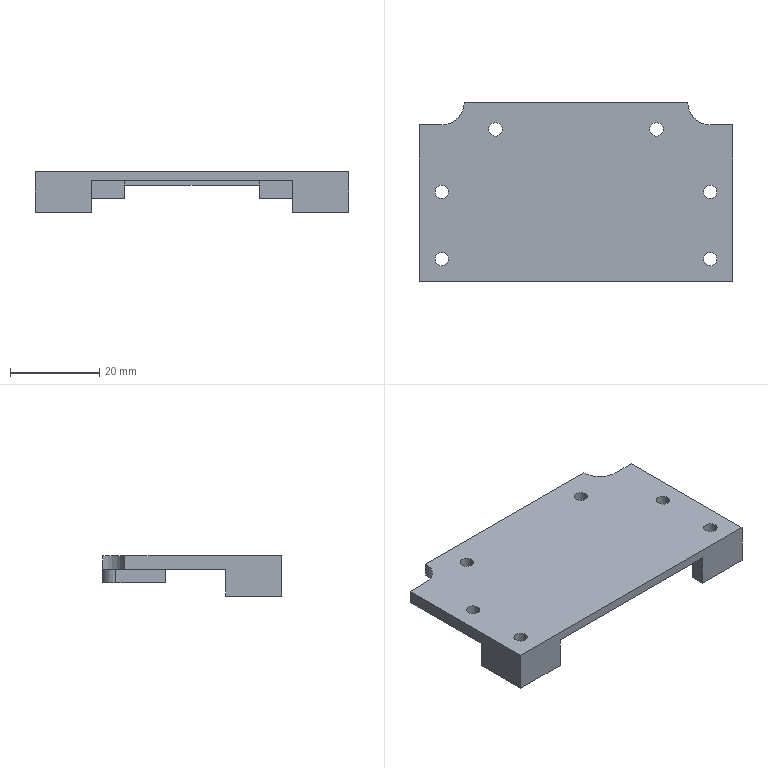Part | SolidWorks | features MBimport 1 | 1 solid | 44 faces | box 70 x 40 x 9 mm | volume 8600 mm3 | plane 28 | cylinder 16 | commonest cylinder face diameters 3 x12 6 x2 10 x2
STEP:
#1=CARTESIAN_POINT('',(-31.5,0.,0.));
#2=VERTEX_POINT('',#1);
#3=CARTESIAN_POINT('',(-28.5,0.,0.));
#4=VERTEX_POINT('',#3);
#5=CARTESIAN_POINT('',(-30.,0.,0.));
#6=DIRECTION('',(0.,0.,1.));
#7=DIRECTION('',(-1.,0.,0.));
#8=AXIS2_PLACEMENT_3D('',#5,#6,#7);
#9=CIRCLE('',#8,1.5);
#10=EDGE_CURVE('',#2,#4,#9,.T.);
#11=ORIENTED_EDGE('',*,*,#10,.T.);
#12=CARTESIAN_POINT('',(-30.,0.,0.));
#13=DIRECTION('',(0.,0.,1.));
#14=DIRECTION('',(1.,0.,0.));
#15=AXIS2_PLACEMENT_3D('',#12,#13,#14);
#16=CIRCLE('',#15,1.5);
#17=EDGE_CURVE('',#4,#2,#16,.T.);
#18=ORIENTED_EDGE('',*,*,#17,.T.);
#19=EDGE_LOOP('',(#11,#18));
#20=FACE_BOUND('',#19,.T.);
#21=CARTESIAN_POINT('',(-25.,6.,0.));
#22=VERTEX_POINT('',#21);
#23=CARTESIAN_POINT('',(-22.5,6.,0.));
#24=VERTEX_POINT('',#23);
#25=CARTESIAN_POINT('',(-25.,6.,0.));
#26=DIRECTION('',(1.,0.,0.));
#27=VECTOR('',#26,1000.);
#28=LINE('',#25,#27);
#29=EDGE_CURVE('',#22,#24,#28,.T.);
#30=ORIENTED_EDGE('',*,*,#29,.T.);
#31=CARTESIAN_POINT('',(-22.5,-17.,0.));
#32=VERTEX_POINT('',#31);
#33=CARTESIAN_POINT('',(-22.5,-17.,0.));
#34=DIRECTION('',(0.,1.,0.));
#35=VECTOR('',#34,1000.);
#36=LINE('',#33,#35);
#37=EDGE_CURVE('',#32,#24,#36,.T.);
#38=ORIENTED_EDGE('',*,*,#37,.F.);
#39=CARTESIAN_POINT('',(-32.,-7.5,0.));
#40=VERTEX_POINT('',#39);
#41=CARTESIAN_POINT('',(-22.5,-17.,0.));
#42=DIRECTION('',(-0.7071,0.7071,0.));
#43=VECTOR('',#42,1000.);
#44=LINE('',#41,#43);
#45=EDGE_CURVE('',#32,#40,#44,.T.);
#46=ORIENTED_EDGE('',*,*,#45,.T.);
#47=CARTESIAN_POINT('',(-35.,-7.5,0.));
#48=VERTEX_POINT('',#47);
#49=CARTESIAN_POINT('',(-35.,-7.5,0.));
#50=DIRECTION('',(1.,0.,0.));
#51=VECTOR('',#50,1000.);
#52=LINE('',#49,#51);
#53=EDGE_CURVE('',#48,#40,#52,.T.);
#54=ORIENTED_EDGE('',*,*,#53,.F.);
#55=CARTESIAN_POINT('',(-35.,15.,0.));
#56=VERTEX_POINT('',#55);
#57=CARTESIAN_POINT('',(-35.,15.,0.));
#58=DIRECTION('',(0.,-1.,0.));
#59=VECTOR('',#58,1000.);
#60=LINE('',#57,#59);
#61=EDGE_CURVE('',#56,#48,#60,.T.);
#62=ORIENTED_EDGE('',*,*,#61,.F.);
#63=CARTESIAN_POINT('',(-30.,15.,0.));
#64=VERTEX_POINT('',#63);
#65=CARTESIAN_POINT('',(-35.,15.,0.));
#66=DIRECTION('',(1.,0.,0.));
#67=VECTOR('',#66,1000.);
#68=LINE('',#65,#67);
#69=EDGE_CURVE('',#56,#64,#68,.T.);
#70=ORIENTED_EDGE('',*,*,#69,.T.);
#71=CARTESIAN_POINT('',(-25.,20.,0.));
#72=VERTEX_POINT('',#71);
#73=CARTESIAN_POINT('',(-30.,20.,0.));
#74=DIRECTION('',(0.,0.,1.));
#75=DIRECTION('',(0.,-1.,0.));
#76=AXIS2_PLACEMENT_3D('',#73,#74,#75);
#77=CIRCLE('',#76,5.);
#78=EDGE_CURVE('',#64,#72,#77,.T.);
#79=ORIENTED_EDGE('',*,*,#78,.T.);
#80=CARTESIAN_POINT('',(-22.,20.,0.));
#81=VERTEX_POINT('',#80);
#82=CARTESIAN_POINT('',(-22.,20.,0.));
#83=DIRECTION('',(-1.,0.,0.));
#84=VECTOR('',#83,1000.);
#85=LINE('',#82,#84);
#86=EDGE_CURVE('',#81,#72,#85,.T.);
#87=ORIENTED_EDGE('',*,*,#86,.F.);
#88=CARTESIAN_POINT('',(-25.,17.,0.));
#89=VERTEX_POINT('',#88);
#90=CARTESIAN_POINT('',(-22.,17.,0.));
#91=DIRECTION('',(0.,0.,1.));
#92=DIRECTION('',(0.,1.,0.));
#93=AXIS2_PLACEMENT_3D('',#90,#91,#92);
#94=CIRCLE('',#93,3.);
#95=EDGE_CURVE('',#81,#89,#94,.T.);
#96=ORIENTED_EDGE('',*,*,#95,.T.);
#97=CARTESIAN_POINT('',(-25.,17.,0.));
#98=DIRECTION('',(0.,-1.,0.));
#99=VECTOR('',#98,1000.);
#100=LINE('',#97,#99);
#101=EDGE_CURVE('',#89,#22,#100,.T.);
#102=ORIENTED_EDGE('',*,*,#101,.T.);
#103=EDGE_LOOP('',(#30,#38,#46,#54,#62,#70,#79,#87,#96,#102));
#104=FACE_OUTER_BOUND('',#103,.T.);
#105=CARTESIAN_POINT('',(0.,0.,0.));
#106=DIRECTION('',(0.,0.,1.));
#107=DIRECTION('',(0.,-1.,0.));
#108=AXIS2_PLACEMENT_3D('',#105,#106,#107);
#109=PLANE('',#108);
#110=ADVANCED_FACE('',(#20,#104),#109,.F.);
#111=ORIENTED_EDGE('',*,*,#10,.F.);
#112=CARTESIAN_POINT('',(-31.5,0.,3.));
#113=VERTEX_POINT('',#112);
#114=CARTESIAN_POINT('',(-31.5,0.,0.));
#115=DIRECTION('',(0.,0.,1.));
#116=VECTOR('',#115,1000.);
#117=LINE('',#114,#116);
#118=EDGE_CURVE('',#2,#113,#117,.T.);
#119=ORIENTED_EDGE('',*,*,#118,.T.);
#120=CARTESIAN_POINT('',(-28.5,0.,3.));
#121=VERTEX_POINT('',#120);
#122=CARTESIAN_POINT('',(-30.,0.,3.));
#123=DIRECTION('',(0.,0.,1.));
#124=DIRECTION('',(-1.,0.,0.));
#125=AXIS2_PLACEMENT_3D('',#122,#123,#124);
#126=CIRCLE('',#125,1.5);
#127=EDGE_CURVE('',#113,#121,#126,.T.);
#128=ORIENTED_EDGE('',*,*,#127,.T.);
#129=CARTESIAN_POINT('',(-28.5,0.,0.));
#130=DIRECTION('',(0.,0.,1.));
#131=VECTOR('',#130,1000.);
#132=LINE('',#129,#131);
#133=EDGE_CURVE('',#4,#121,#132,.T.);
#134=ORIENTED_EDGE('',*,*,#133,.F.);
#135=EDGE_LOOP('',(#111,#119,#128,#134));
#136=FACE_OUTER_BOUND('',#135,.T.);
#137=CARTESIAN_POINT('',(-30.,0.,0.));
#138=DIRECTION('',(0.,0.,-1.));
#139=DIRECTION('',(1.,0.,0.));
#140=AXIS2_PLACEMENT_3D('',#137,#138,#139);
#141=CYLINDRICAL_SURFACE('',#140,1.5);
#142=ADVANCED_FACE('',(#136),#141,.F.);
#143=CARTESIAN_POINT('',(-30.,0.,3.));
#144=DIRECTION('',(0.,0.,1.));
#145=DIRECTION('',(1.,0.,0.));
#146=AXIS2_PLACEMENT_3D('',#143,#144,#145);
#147=CIRCLE('',#146,1.5);
#148=EDGE_CURVE('',#121,#113,#147,.T.);
#149=ORIENTED_EDGE('',*,*,#148,.T.);
#150=ORIENTED_EDGE('',*,*,#118,.F.);
#151=ORIENTED_EDGE('',*,*,#17,.F.);
#152=ORIENTED_EDGE('',*,*,#133,.T.);
#153=EDGE_LOOP('',(#149,#150,#151,#152));
#154=FACE_OUTER_BOUND('',#153,.T.);
#155=CARTESIAN_POINT('',(-30.,0.,0.));
#156=DIRECTION('',(0.,0.,-1.));
#157=DIRECTION('',(1.,0.,0.));
#158=AXIS2_PLACEMENT_3D('',#155,#156,#157);
#159=CYLINDRICAL_SURFACE('',#158,1.5);
#160=ADVANCED_FACE('',(#154),#159,.F.);
#161=CARTESIAN_POINT('',(-25.,6.,-3.));
#162=VERTEX_POINT('',#161);
#163=CARTESIAN_POINT('',(-15.,6.,-3.));
#164=VERTEX_POINT('',#163);
#165=CARTESIAN_POINT('',(-25.,6.,-3.));
#166=DIRECTION('',(1.,0.,0.));
#167=VECTOR('',#166,1000.);
#168=LINE('',#165,#167);
#169=EDGE_CURVE('',#162,#164,#168,.T.);
#170=ORIENTED_EDGE('',*,*,#169,.T.);
#171=CARTESIAN_POINT('',(-15.,6.,1.));
#172=VERTEX_POINT('',#171);
#173=CARTESIAN_POINT('',(-15.,6.,1.));
#174=DIRECTION('',(0.,0.,-1.));
#175=VECTOR('',#174,1000.);
#176=LINE('',#173,#175);
#177=EDGE_CURVE('',#172,#164,#176,.T.);
#178=ORIENTED_EDGE('',*,*,#177,.F.);
#179=CARTESIAN_POINT('',(-22.5,6.,1.));
#180=VERTEX_POINT('',#179);
#181=CARTESIAN_POINT('',(-22.5,6.,1.));
#182=DIRECTION('',(1.,0.,0.));
#183=VECTOR('',#182,1000.);
#184=LINE('',#181,#183);
#185=EDGE_CURVE('',#180,#172,#184,.T.);
#186=ORIENTED_EDGE('',*,*,#185,.F.);
#187=CARTESIAN_POINT('',(-22.5,6.,1.));
#188=DIRECTION('',(0.,0.,-1.));
#189=VECTOR('',#188,1000.);
#190=LINE('',#187,#189);
#191=EDGE_CURVE('',#180,#24,#190,.T.);
#192=ORIENTED_EDGE('',*,*,#191,.T.);
#193=ORIENTED_EDGE('',*,*,#29,.F.);
#194=CARTESIAN_POINT('',(-25.,6.,0.));
#195=DIRECTION('',(0.,0.,-1.));
#196=VECTOR('',#195,1000.);
#197=LINE('',#194,#196);
#198=EDGE_CURVE('',#22,#162,#197,.T.);
#199=ORIENTED_EDGE('',*,*,#198,.T.);
#200=EDGE_LOOP('',(#170,#178,#186,#192,#193,#199));
#201=FACE_OUTER_BOUND('',#200,.T.);
#202=CARTESIAN_POINT('',(-25.,6.,1.));
#203=DIRECTION('',(0.,1.,0.));
#204=DIRECTION('',(1.,0.,0.));
#205=AXIS2_PLACEMENT_3D('',#202,#203,#204);
#206=PLANE('',#205);
#207=ADVANCED_FACE('',(#201),#206,.F.);
#208=CARTESIAN_POINT('',(-22.5,-20.,1.));
#209=VERTEX_POINT('',#208);
#210=CARTESIAN_POINT('',(-22.5,-20.,1.));
#211=DIRECTION('',(0.,1.,0.));
#212=VECTOR('',#211,1000.);
#213=LINE('',#210,#212);
#214=EDGE_CURVE('',#209,#180,#213,.T.);
#215=ORIENTED_EDGE('',*,*,#214,.F.);
#216=CARTESIAN_POINT('',(-22.5,-20.,-6.));
#217=VERTEX_POINT('',#216);
#218=CARTESIAN_POINT('',(-22.5,-20.,-6.));
#219=DIRECTION('',(0.,0.,1.));
#220=VECTOR('',#219,1000.);
#221=LINE('',#218,#220);
#222=EDGE_CURVE('',#217,#209,#221,.T.);
#223=ORIENTED_EDGE('',*,*,#222,.F.);
#224=CARTESIAN_POINT('',(-22.5,-17.,-6.));
#225=VERTEX_POINT('',#224);
#226=CARTESIAN_POINT('',(-22.5,-20.,-6.));
#227=DIRECTION('',(0.,1.,0.));
#228=VECTOR('',#227,1000.);
#229=LINE('',#226,#228);
#230=EDGE_CURVE('',#217,#225,#229,.T.);
#231=ORIENTED_EDGE('',*,*,#230,.T.);
#232=CARTESIAN_POINT('',(-22.5,-17.,0.));
#233=DIRECTION('',(0.,0.,-1.));
#234=VECTOR('',#233,1000.);
#235=LINE('',#232,#234);
#236=EDGE_CURVE('',#32,#225,#235,.T.);
#237=ORIENTED_EDGE('',*,*,#236,.F.);
#238=ORIENTED_EDGE('',*,*,#37,.T.);
#239=ORIENTED_EDGE('',*,*,#191,.F.);
#240=EDGE_LOOP('',(#215,#223,#231,#237,#238,#239));
#241=FACE_OUTER_BOUND('',#240,.T.);
#242=CARTESIAN_POINT('',(-22.5,-20.,0.));
#243=DIRECTION('',(-1.,0.,0.));
#244=DIRECTION('',(0.,1.,0.));
#245=AXIS2_PLACEMENT_3D('',#242,#243,#244);
#246=PLANE('',#245);
#247=ADVANCED_FACE('',(#241),#246,.F.);
#248=CARTESIAN_POINT('',(-32.,-7.5,-6.));
#249=VERTEX_POINT('',#248);
#250=CARTESIAN_POINT('',(-22.5,-17.,-6.));
#251=DIRECTION('',(-0.7071,0.7071,0.));
#252=VECTOR('',#251,1000.);
#253=LINE('',#250,#252);
#254=EDGE_CURVE('',#225,#249,#253,.T.);
#255=ORIENTED_EDGE('',*,*,#254,.T.);
#256=CARTESIAN_POINT('',(-32.,-7.5,0.));
#257=DIRECTION('',(0.,0.,-1.));
#258=VECTOR('',#257,1000.);
#259=LINE('',#256,#258);
#260=EDGE_CURVE('',#40,#249,#259,.T.);
#261=ORIENTED_EDGE('',*,*,#260,.F.);
#262=ORIENTED_EDGE('',*,*,#45,.F.);
#263=ORIENTED_EDGE('',*,*,#236,.T.);
#264=EDGE_LOOP('',(#255,#261,#262,#263));
#265=FACE_OUTER_BOUND('',#264,.T.);
#266=CARTESIAN_POINT('',(-22.5,-17.,0.));
#267=DIRECTION('',(-0.7071,-0.7071,0.));
#268=DIRECTION('',(-0.7071,0.7071,0.));
#269=AXIS2_PLACEMENT_3D('',#266,#267,#268);
#270=PLANE('',#269);
#271=ADVANCED_FACE('',(#265),#270,.F.);
#272=CARTESIAN_POINT('',(-35.,-7.5,-6.));
#273=VERTEX_POINT('',#272);
#274=CARTESIAN_POINT('',(-32.,-7.5,-6.));
#275=DIRECTION('',(-1.,0.,0.));
#276=VECTOR('',#275,1000.);
#277=LINE('',#274,#276);
#278=EDGE_CURVE('',#249,#273,#277,.T.);
#279=ORIENTED_EDGE('',*,*,#278,.T.);
#280=CARTESIAN_POINT('',(-35.,-7.5,0.));
#281=DIRECTION('',(0.,0.,-1.));
#282=VECTOR('',#281,1000.);
#283=LINE('',#280,#282);
#284=EDGE_CURVE('',#48,#273,#283,.T.);
#285=ORIENTED_EDGE('',*,*,#284,.F.);
#286=ORIENTED_EDGE('',*,*,#53,.T.);
#287=ORIENTED_EDGE('',*,*,#260,.T.);
#288=EDGE_LOOP('',(#279,#285,#286,#287));
#289=FACE_OUTER_BOUND('',#288,.T.);
#290=CARTESIAN_POINT('',(-32.,-7.5,0.));
#291=DIRECTION('',(0.,-1.,0.));
#292=DIRECTION('',(-1.,0.,0.));
#293=AXIS2_PLACEMENT_3D('',#290,#291,#292);
#294=PLANE('',#293);
#295=ADVANCED_FACE('',(#289),#294,.F.);
#296=ORIENTED_EDGE('',*,*,#61,.T.);
#297=ORIENTED_EDGE('',*,*,#284,.T.);
#298=CARTESIAN_POINT('',(-35.,-20.,-6.));
#299=VERTEX_POINT('',#298);
#300=CARTESIAN_POINT('',(-35.,-7.5,-6.));
#301=DIRECTION('',(0.,-1.,0.));
#302=VECTOR('',#301,1000.);
#303=LINE('',#300,#302);
#304=EDGE_CURVE('',#273,#299,#303,.T.);
#305=ORIENTED_EDGE('',*,*,#304,.T.);
#306=CARTESIAN_POINT('',(-35.,-20.,3.));
#307=VERTEX_POINT('',#306);
#308=CARTESIAN_POINT('',(-35.,-20.,3.));
#309=DIRECTION('',(0.,0.,-1.));
#310=VECTOR('',#309,1000.);
#311=LINE('',#308,#310);
#312=EDGE_CURVE('',#307,#299,#311,.T.);
#313=ORIENTED_EDGE('',*,*,#312,.F.);
#314=CARTESIAN_POINT('',(-35.,15.,3.));
#315=VERTEX_POINT('',#314);
#316=CARTESIAN_POINT('',(-35.,15.,3.));
#317=DIRECTION('',(0.,-1.,0.));
#318=VECTOR('',#317,1000.);
#319=LINE('',#316,#318);
#320=EDGE_CURVE('',#315,#307,#319,.T.);
#321=ORIENTED_EDGE('',*,*,#320,.F.);
#322=CARTESIAN_POINT('',(-35.,15.,3.));
#323=DIRECTION('',(0.,0.,-1.));
#324=VECTOR('',#323,1000.);
#325=LINE('',#322,#324);
#326=EDGE_CURVE('',#315,#56,#325,.T.);
#327=ORIENTED_EDGE('',*,*,#326,.T.);
#328=EDGE_LOOP('',(#296,#297,#305,#313,#321,#327));
#329=FACE_OUTER_BOUND('',#328,.T.);
#330=CARTESIAN_POINT('',(-35.,20.,0.));
#331=DIRECTION('',(-1.,0.,0.));
#332=DIRECTION('',(0.,-1.,0.));
#333=AXIS2_PLACEMENT_3D('',#330,#331,#332);
#334=PLANE('',#333);
#335=ADVANCED_FACE('',(#329),#334,.T.);
#336=ORIENTED_EDGE('',*,*,#69,.F.);
#337=ORIENTED_EDGE('',*,*,#326,.F.);
#338=CARTESIAN_POINT('',(-30.,15.,3.));
#339=VERTEX_POINT('',#338);
#340=CARTESIAN_POINT('',(-35.,15.,3.));
#341=DIRECTION('',(1.,0.,0.));
#342=VECTOR('',#341,1000.);
#343=LINE('',#340,#342);
#344=EDGE_CURVE('',#315,#339,#343,.T.);
#345=ORIENTED_EDGE('',*,*,#344,.T.);
#346=CARTESIAN_POINT('',(-30.,15.,3.));
#347=DIRECTION('',(0.,0.,-1.));
#348=VECTOR('',#347,1000.);
#349=LINE('',#346,#348);
#350=EDGE_CURVE('',#339,#64,#349,.T.);
#351=ORIENTED_EDGE('',*,*,#350,.T.);
#352=EDGE_LOOP('',(#336,#337,#345,#351));
#353=FACE_OUTER_BOUND('',#352,.T.);
#354=CARTESIAN_POINT('',(-35.,15.,0.));
#355=DIRECTION('',(0.,1.,0.));
#356=DIRECTION('',(1.,0.,0.));
#357=AXIS2_PLACEMENT_3D('',#354,#355,#356);
#358=PLANE('',#357);
#359=ADVANCED_FACE('',(#353),#358,.T.);
#360=ORIENTED_EDGE('',*,*,#350,.F.);
#361=CARTESIAN_POINT('',(-25.,20.,3.));
#362=VERTEX_POINT('',#361);
#363=CARTESIAN_POINT('',(-30.,20.,3.));
#364=DIRECTION('',(0.,0.,-1.));
#365=DIRECTION('',(1.,0.,0.));
#366=AXIS2_PLACEMENT_3D('',#363,#364,#365);
#367=CIRCLE('',#366,5.);
#368=EDGE_CURVE('',#362,#339,#367,.T.);
#369=ORIENTED_EDGE('',*,*,#368,.F.);
#370=CARTESIAN_POINT('',(-25.,20.,3.));
#371=DIRECTION('',(0.,0.,-1.));
#372=VECTOR('',#371,1000.);
#373=LINE('',#370,#372);
#374=EDGE_CURVE('',#362,#72,#373,.T.);
#375=ORIENTED_EDGE('',*,*,#374,.T.);
#376=ORIENTED_EDGE('',*,*,#78,.F.);
#377=EDGE_LOOP('',(#360,#369,#375,#376));
#378=FACE_OUTER_BOUND('',#377,.T.);
#379=CARTESIAN_POINT('',(-30.,20.,14.732));
#380=DIRECTION('',(0.,0.,1.));
#381=DIRECTION('',(1.,0.,0.));
#382=AXIS2_PLACEMENT_3D('',#379,#380,#381);
#383=CYLINDRICAL_SURFACE('',#382,5.);
#384=ADVANCED_FACE('',(#378),#383,.F.);
#385=CARTESIAN_POINT('',(-22.,20.,-3.));
#386=VERTEX_POINT('',#385);
#387=CARTESIAN_POINT('',(-22.,20.,0.));
#388=DIRECTION('',(0.,0.,-1.));
#389=VECTOR('',#388,1000.);
#390=LINE('',#387,#389);
#391=EDGE_CURVE('',#81,#386,#390,.T.);
#392=ORIENTED_EDGE('',*,*,#391,.F.);
#393=ORIENTED_EDGE('',*,*,#86,.T.);
#394=ORIENTED_EDGE('',*,*,#374,.F.);
#395=CARTESIAN_POINT('',(25.,20.,3.));
#396=VERTEX_POINT('',#395);
#397=CARTESIAN_POINT('',(25.,20.,3.));
#398=DIRECTION('',(-1.,0.,0.));
#399=VECTOR('',#398,1000.);
#400=LINE('',#397,#399);
#401=EDGE_CURVE('',#396,#362,#400,.T.);
#402=ORIENTED_EDGE('',*,*,#401,.F.);
#403=CARTESIAN_POINT('',(25.,20.,0.));
#404=VERTEX_POINT('',#403);
#405=CARTESIAN_POINT('',(25.,20.,0.));
#406=DIRECTION('',(0.,0.,1.));
#407=VECTOR('',#406,1000.);
#408=LINE('',#405,#407);
#409=EDGE_CURVE('',#404,#396,#408,.T.);
#410=ORIENTED_EDGE('',*,*,#409,.F.);
#411=CARTESIAN_POINT('',(22.,20.,0.));
#412=VERTEX_POINT('',#411);
#413=CARTESIAN_POINT('',(22.,20.,0.));
#414=DIRECTION('',(1.,0.,0.));
#415=VECTOR('',#414,1000.);
#416=LINE('',#413,#415);
#417=EDGE_CURVE('',#412,#404,#416,.T.);
#418=ORIENTED_EDGE('',*,*,#417,.F.);
#419=CARTESIAN_POINT('',(22.,20.,-3.));
#420=VERTEX_POINT('',#419);
#421=CARTESIAN_POINT('',(22.,20.,-3.));
#422=DIRECTION('',(0.,0.,1.));
#423=VECTOR('',#422,1000.);
#424=LINE('',#421,#423);
#425=EDGE_CURVE('',#420,#412,#424,.T.);
#426=ORIENTED_EDGE('',*,*,#425,.F.);
#427=CARTESIAN_POINT('',(15.,20.,-3.));
#428=VERTEX_POINT('',#427);
#429=CARTESIAN_POINT('',(15.,20.,-3.));
#430=DIRECTION('',(1.,0.,0.));
#431=VECTOR('',#430,1000.);
#432=LINE('',#429,#431);
#433=EDGE_CURVE('',#428,#420,#432,.T.);
#434=ORIENTED_EDGE('',*,*,#433,.F.);
#435=CARTESIAN_POINT('',(15.,20.,0.));
#436=VERTEX_POINT('',#435);
#437=CARTESIAN_POINT('',(15.,20.,0.));
#438=DIRECTION('',(0.,0.,-1.));
#439=VECTOR('',#438,1000.);
#440=LINE('',#437,#439);
#441=EDGE_CURVE('',#436,#428,#440,.T.);
#442=ORIENTED_EDGE('',*,*,#441,.F.);
#443=CARTESIAN_POINT('',(-15.,20.,0.));
#444=VERTEX_POINT('',#443);
#445=CARTESIAN_POINT('',(15.,20.,0.));
#446=DIRECTION('',(-1.,0.,0.));
#447=VECTOR('',#446,1000.);
#448=LINE('',#445,#447);
#449=EDGE_CURVE('',#436,#444,#448,.T.);
#450=ORIENTED_EDGE('',*,*,#449,.T.);
#451=CARTESIAN_POINT('',(-15.,20.,-3.));
#452=VERTEX_POINT('',#451);
#453=CARTESIAN_POINT('',(-15.,20.,0.));
#454=DIRECTION('',(0.,0.,-1.));
#455=VECTOR('',#454,1000.);
#456=LINE('',#453,#455);
#457=EDGE_CURVE('',#444,#452,#456,.T.);
#458=ORIENTED_EDGE('',*,*,#457,.T.);
#459=CARTESIAN_POINT('',(-15.,20.,-3.));
#460=DIRECTION('',(-1.,0.,0.));
#461=VECTOR('',#460,1000.);
#462=LINE('',#459,#461);
#463=EDGE_CURVE('',#452,#386,#462,.T.);
#464=ORIENTED_EDGE('',*,*,#463,.T.);
#465=EDGE_LOOP('',(#392,#393,#394,#402,#410,#418,#426,#434,#442,#450,#458,#464));
#466=FACE_OUTER_BOUND('',#465,.T.);
#467=CARTESIAN_POINT('',(35.,20.,0.));
#468=DIRECTION('',(0.,1.,0.));
#469=DIRECTION('',(-1.,0.,0.));
#470=AXIS2_PLACEMENT_3D('',#467,#468,#469);
#471=PLANE('',#470);
#472=ADVANCED_FACE('',(#466),#471,.T.);
#473=CARTESIAN_POINT('',(-25.,17.,-3.));
#474=VERTEX_POINT('',#473);
#475=CARTESIAN_POINT('',(-25.,17.,0.));
#476=DIRECTION('',(0.,0.,-1.));
#477=VECTOR('',#476,1000.);
#478=LINE('',#475,#477);
#479=EDGE_CURVE('',#89,#474,#478,.T.);
#480=ORIENTED_EDGE('',*,*,#479,.F.);
#481=ORIENTED_EDGE('',*,*,#95,.F.);
#482=ORIENTED_EDGE('',*,*,#391,.T.);
#483=CARTESIAN_POINT('',(-22.,17.,-3.));
#484=DIRECTION('',(0.,0.,-1.));
#485=DIRECTION('',(-1.,0.,0.));
#486=AXIS2_PLACEMENT_3D('',#483,#484,#485);
#487=CIRCLE('',#486,3.);
#488=EDGE_CURVE('',#474,#386,#487,.T.);
#489=ORIENTED_EDGE('',*,*,#488,.F.);
#490=EDGE_LOOP('',(#480,#481,#482,#489));
#491=FACE_OUTER_BOUND('',#490,.T.);
#492=CARTESIAN_POINT('',(-22.,17.,14.732));
#493=DIRECTION('',(0.,0.,1.));
#494=DIRECTION('',(-1.,0.,0.));
#495=AXIS2_PLACEMENT_3D('',#492,#493,#494);
#496=CYLINDRICAL_SURFACE('',#495,3.);
#497=ADVANCED_FACE('',(#491),#496,.T.);
#498=ORIENTED_EDGE('',*,*,#198,.F.);
#499=ORIENTED_EDGE('',*,*,#101,.F.);
#500=ORIENTED_EDGE('',*,*,#479,.T.);
#501=CARTESIAN_POINT('',(-25.,17.,-3.));
#502=DIRECTION('',(0.,-1.,0.));
#503=VECTOR('',#502,1000.);
#504=LINE('',#501,#503);
#505=EDGE_CURVE('',#474,#162,#504,.T.);
#506=ORIENTED_EDGE('',*,*,#505,.T.);
#507=EDGE_LOOP('',(#498,#499,#500,#506));
#508=FACE_OUTER_BOUND('',#507,.T.);
#509=CARTESIAN_POINT('',(-25.,20.,1.));
#510=DIRECTION('',(1.,0.,0.));
#511=DIRECTION('',(0.,-1.,0.));
#512=AXIS2_PLACEMENT_3D('',#509,#510,#511);
#513=PLANE('',#512);
#514=ADVANCED_FACE('',(#508),#513,.F.);
#515=CARTESIAN_POINT('',(-19.5,14.,3.));
#516=VERTEX_POINT('',#515);
#517=CARTESIAN_POINT('',(-16.5,14.,3.));
#518=VERTEX_POINT('',#517);
#519=CARTESIAN_POINT('',(-18.,14.,3.));
#520=DIRECTION('',(0.,0.,1.));
#521=DIRECTION('',(-1.,0.,0.));
#522=AXIS2_PLACEMENT_3D('',#519,#520,#521);
#523=CIRCLE('',#522,1.5);
#524=EDGE_CURVE('',#516,#518,#523,.T.);
#525=ORIENTED_EDGE('',*,*,#524,.F.);
#526=CARTESIAN_POINT('',(-18.,14.,3.));
#527=DIRECTION('',(0.,0.,1.));
#528=DIRECTION('',(1.,0.,0.));
#529=AXIS2_PLACEMENT_3D('',#526,#527,#528);
#530=CIRCLE('',#529,1.5);
#531=EDGE_CURVE('',#518,#516,#530,.T.);
#532=ORIENTED_EDGE('',*,*,#531,.F.);
#533=EDGE_LOOP('',(#525,#532));
#534=FACE_BOUND('',#533,.T.);
#535=CARTESIAN_POINT('',(19.5,14.,3.));
#536=VERTEX_POINT('',#535);
#537=CARTESIAN_POINT('',(16.5,14.,3.));
#538=VERTEX_POINT('',#537);
#539=CARTESIAN_POINT('',(18.,14.,3.));
#540=DIRECTION('',(0.,0.,-1.));
#541=DIRECTION('',(1.,0.,0.));
#542=AXIS2_PLACEMENT_3D('',#539,#540,#541);
#543=CIRCLE('',#542,1.5);
#544=EDGE_CURVE('',#536,#538,#543,.T.);
#545=ORIENTED_EDGE('',*,*,#544,.T.);
#546=CARTESIAN_POINT('',(18.,14.,3.));
#547=DIRECTION('',(0.,0.,-1.));
#548=DIRECTION('',(-1.,0.,0.));
#549=AXIS2_PLACEMENT_3D('',#546,#547,#548);
#550=CIRCLE('',#549,1.5);
#551=EDGE_CURVE('',#538,#536,#550,.T.);
#552=ORIENTED_EDGE('',*,*,#551,.T.);
#553=EDGE_LOOP('',(#545,#552));
#554=FACE_BOUND('',#553,.T.);
#555=ORIENTED_EDGE('',*,*,#127,.F.);
#556=ORIENTED_EDGE('',*,*,#148,.F.);
#557=EDGE_LOOP('',(#555,#556));
#558=FACE_BOUND('',#557,.T.);
#559=CARTESIAN_POINT('',(31.5,0.,3.));
#560=VERTEX_POINT('',#559);
#561=CARTESIAN_POINT('',(28.5,0.,3.));
#562=VERTEX_POINT('',#561);
#563=CARTESIAN_POINT('',(30.,0.,3.));
#564=DIRECTION('',(0.,0.,-1.));
#565=DIRECTION('',(1.,0.,0.));
#566=AXIS2_PLACEMENT_3D('',#563,#564,#565);
#567=CIRCLE('',#566,1.5);
#568=EDGE_CURVE('',#560,#562,#567,.T.);
#569=ORIENTED_EDGE('',*,*,#568,.T.);
#570=CARTESIAN_POINT('',(30.,0.,3.));
#571=DIRECTION('',(0.,0.,-1.));
#572=DIRECTION('',(-1.,0.,0.));
#573=AXIS2_PLACEMENT_3D('',#570,#571,#572);
#574=CIRCLE('',#573,1.5);
#575=EDGE_CURVE('',#562,#560,#574,.T.);
#576=ORIENTED_EDGE('',*,*,#575,.T.);
#577=EDGE_LOOP('',(#569,#576));
#578=FACE_BOUND('',#577,.T.);
#579=ORIENTED_EDGE('',*,*,#320,.T.);
#580=CARTESIAN_POINT('',(35.,-20.,3.));
#581=VERTEX_POINT('',#580);
#582=CARTESIAN_POINT('',(-35.,-20.,3.));
#583=DIRECTION('',(1.,0.,0.));
#584=VECTOR('',#583,1000.);
#585=LINE('',#582,#584);
#586=EDGE_CURVE('',#307,#581,#585,.T.);
#587=ORIENTED_EDGE('',*,*,#586,.T.);
#588=CARTESIAN_POINT('',(35.,15.,3.));
#589=VERTEX_POINT('',#588);
#590=CARTESIAN_POINT('',(35.,-20.,3.));
#591=DIRECTION('',(0.,1.,0.));
#592=VECTOR('',#591,1000.);
#593=LINE('',#590,#592);
#594=EDGE_CURVE('',#581,#589,#593,.T.);
#595=ORIENTED_EDGE('',*,*,#594,.T.);
#596=CARTESIAN_POINT('',(30.,15.,3.));
#597=VERTEX_POINT('',#596);
#598=CARTESIAN_POINT('',(35.,15.,3.));
#599=DIRECTION('',(-1.,0.,0.));
#600=VECTOR('',#599,1000.);
#601=LINE('',#598,#600);
#602=EDGE_CURVE('',#589,#597,#601,.T.);
#603=ORIENTED_EDGE('',*,*,#602,.T.);
#604=CARTESIAN_POINT('',(30.,20.,3.));
#605=DIRECTION('',(0.,0.,-1.));
#606=DIRECTION('',(0.,-1.,0.));
#607=AXIS2_PLACEMENT_3D('',#604,#605,#606);
#608=CIRCLE('',#607,5.);
#609=EDGE_CURVE('',#597,#396,#608,.T.);
#610=ORIENTED_EDGE('',*,*,#609,.T.);
#611=ORIENTED_EDGE('',*,*,#401,.T.);
#612=ORIENTED_EDGE('',*,*,#368,.T.);
#613=ORIENTED_EDGE('',*,*,#344,.F.);
#614=EDGE_LOOP('',(#579,#587,#595,#603,#610,#611,#612,#613));
#615=FACE_OUTER_BOUND('',#614,.T.);
#616=CARTESIAN_POINT('',(-31.5,-15.,3.));
#617=VERTEX_POINT('',#616);
#618=CARTESIAN_POINT('',(-28.5,-15.,3.));
#619=VERTEX_POINT('',#618);
#620=CARTESIAN_POINT('',(-30.,-15.,3.));
#621=DIRECTION('',(0.,0.,1.));
#622=DIRECTION('',(-1.,0.,0.));
#623=AXIS2_PLACEMENT_3D('',#620,#621,#622);
#624=CIRCLE('',#623,1.5);
#625=EDGE_CURVE('',#617,#619,#624,.T.);
#626=ORIENTED_EDGE('',*,*,#625,.F.);
#627=CARTESIAN_POINT('',(-30.,-15.,3.));
#628=DIRECTION('',(0.,0.,1.));
#629=DIRECTION('',(1.,0.,0.));
#630=AXIS2_PLACEMENT_3D('',#627,#628,#629);
#631=CIRCLE('',#630,1.5);
#632=EDGE_CURVE('',#619,#617,#631,.T.);
#633=ORIENTED_EDGE('',*,*,#632,.F.);
#634=EDGE_LOOP('',(#626,#633));
#635=FACE_BOUND('',#634,.T.);
#636=CARTESIAN_POINT('',(31.5,-15.,3.));
#637=VERTEX_POINT('',#636);
#638=CARTESIAN_POINT('',(28.5,-15.,3.));
#639=VERTEX_POINT('',#638);
#640=CARTESIAN_POINT('',(30.,-15.,3.));
#641=DIRECTION('',(0.,0.,-1.));
#642=DIRECTION('',(1.,0.,0.));
#643=AXIS2_PLACEMENT_3D('',#640,#641,#642);
#644=CIRCLE('',#643,1.5);
#645=EDGE_CURVE('',#637,#639,#644,.T.);
#646=ORIENTED_EDGE('',*,*,#645,.T.);
#647=CARTESIAN_POINT('',(30.,-15.,3.));
#648=DIRECTION('',(0.,0.,-1.));
#649=DIRECTION('',(-1.,0.,0.));
#650=AXIS2_PLACEMENT_3D('',#647,#648,#649);
#651=CIRCLE('',#650,1.5);
#652=EDGE_CURVE('',#639,#637,#651,.T.);
#653=ORIENTED_EDGE('',*,*,#652,.T.);
#654=EDGE_LOOP('',(#646,#653));
#655=FACE_BOUND('',#654,.T.);
#656=CARTESIAN_POINT('',(0.,0.,3.));
#657=DIRECTION('',(0.,0.,1.));
#658=DIRECTION('',(0.,-1.,0.));
#659=AXIS2_PLACEMENT_3D('',#656,#657,#658);
#660=PLANE('',#659);
#661=ADVANCED_FACE('',(#534,#554,#558,#578,#615,#635,#655),#660,.T.);
#662=CARTESIAN_POINT('',(-19.5,14.,-3.));
#663=VERTEX_POINT('',#662);
#664=CARTESIAN_POINT('',(-16.5,14.,-3.));
#665=VERTEX_POINT('',#664);
#666=CARTESIAN_POINT('',(-18.,14.,-3.));
#667=DIRECTION('',(0.,0.,1.));
#668=DIRECTION('',(-1.,0.,0.));
#669=AXIS2_PLACEMENT_3D('',#666,#667,#668);
#670=CIRCLE('',#669,1.5);
#671=EDGE_CURVE('',#663,#665,#670,.T.);
#672=ORIENTED_EDGE('',*,*,#671,.T.);
#673=CARTESIAN_POINT('',(-18.,14.,-3.));
#674=DIRECTION('',(0.,0.,1.));
#675=DIRECTION('',(1.,0.,0.));
#676=AXIS2_PLACEMENT_3D('',#673,#674,#675);
#677=CIRCLE('',#676,1.5);
#678=EDGE_CURVE('',#665,#663,#677,.T.);
#679=ORIENTED_EDGE('',*,*,#678,.T.);
#680=EDGE_LOOP('',(#672,#679));
#681=FACE_BOUND('',#680,.T.);
#682=CARTESIAN_POINT('',(-15.,6.,-3.));
#683=DIRECTION('',(0.,1.,0.));
#684=VECTOR('',#683,1000.);
#685=LINE('',#682,#684);
#686=EDGE_CURVE('',#164,#452,#685,.T.);
#687=ORIENTED_EDGE('',*,*,#686,.F.);
#688=ORIENTED_EDGE('',*,*,#169,.F.);
#689=ORIENTED_EDGE('',*,*,#505,.F.);
#690=ORIENTED_EDGE('',*,*,#488,.T.);
#691=ORIENTED_EDGE('',*,*,#463,.F.);
#692=EDGE_LOOP('',(#687,#688,#689,#690,#691));
#693=FACE_OUTER_BOUND('',#692,.T.);
#694=CARTESIAN_POINT('',(0.,0.,-3.));
#695=DIRECTION('',(0.,0.,1.));
#696=DIRECTION('',(1.,0.,0.));
#697=AXIS2_PLACEMENT_3D('',#694,#695,#696);
#698=PLANE('',#697);
#699=ADVANCED_FACE('',(#681,#693),#698,.F.);
#700=CARTESIAN_POINT('',(-15.,15.,0.));
#701=VERTEX_POINT('',#700);
#702=CARTESIAN_POINT('',(-15.,20.,0.));
#703=DIRECTION('',(0.,-1.,0.));
#704=VECTOR('',#703,1000.);
#705=LINE('',#702,#704);
#706=EDGE_CURVE('',#444,#701,#705,.T.);
#707=ORIENTED_EDGE('',*,*,#706,.T.);
#708=CARTESIAN_POINT('',(-15.,15.,1.));
#709=VERTEX_POINT('',#708);
#710=CARTESIAN_POINT('',(-15.,15.,1.));
#711=DIRECTION('',(0.,0.,-1.));
#712=VECTOR('',#711,1000.);
#713=LINE('',#710,#712);
#714=EDGE_CURVE('',#709,#701,#713,.T.);
#715=ORIENTED_EDGE('',*,*,#714,.F.);
#716=CARTESIAN_POINT('',(-15.,15.,1.));
#717=DIRECTION('',(0.,-1.,0.));
#718=VECTOR('',#717,1000.);
#719=LINE('',#716,#718);
#720=EDGE_CURVE('',#709,#172,#719,.T.);
#721=ORIENTED_EDGE('',*,*,#720,.T.);
#722=ORIENTED_EDGE('',*,*,#177,.T.);
#723=ORIENTED_EDGE('',*,*,#686,.T.);
#724=ORIENTED_EDGE('',*,*,#457,.F.);
#725=EDGE_LOOP('',(#707,#715,#721,#722,#723,#724));
#726=FACE_OUTER_BOUND('',#725,.T.);
#727=CARTESIAN_POINT('',(-15.,6.,1.));
#728=DIRECTION('',(-1.,0.,0.));
#729=DIRECTION('',(0.,1.,0.));
#730=AXIS2_PLACEMENT_3D('',#727,#728,#729);
#731=PLANE('',#730);
#732=ADVANCED_FACE('',(#726),#731,.F.);
#733=ORIENTED_EDGE('',*,*,#720,.F.);
#734=CARTESIAN_POINT('',(15.,15.,1.));
#735=VERTEX_POINT('',#734);
#736=CARTESIAN_POINT('',(-15.,15.,1.));
#737=DIRECTION('',(1.,0.,0.));
#738=VECTOR('',#737,1000.);
#739=LINE('',#736,#738);
#740=EDGE_CURVE('',#709,#735,#739,.T.);
#741=ORIENTED_EDGE('',*,*,#740,.T.);
#742=CARTESIAN_POINT('',(15.,6.,1.));
#743=VERTEX_POINT('',#742);
#744=CARTESIAN_POINT('',(15.,15.,1.));
#745=DIRECTION('',(0.,-1.,0.));
#746=VECTOR('',#745,1000.);
#747=LINE('',#744,#746);
#748=EDGE_CURVE('',#735,#743,#747,.T.);
#749=ORIENTED_EDGE('',*,*,#748,.T.);
#750=CARTESIAN_POINT('',(22.5,6.,1.));
#751=VERTEX_POINT('',#750);
#752=CARTESIAN_POINT('',(22.5,6.,1.));
#753=DIRECTION('',(-1.,0.,0.));
#754=VECTOR('',#753,1000.);
#755=LINE('',#752,#754);
#756=EDGE_CURVE('',#751,#743,#755,.T.);
#757=ORIENTED_EDGE('',*,*,#756,.F.);
#758=CARTESIAN_POINT('',(22.5,-20.,1.));
#759=VERTEX_POINT('',#758);
#760=CARTESIAN_POINT('',(22.5,6.,1.));
#761=DIRECTION('',(0.,-1.,0.));
#762=VECTOR('',#761,1000.);
#763=LINE('',#760,#762);
#764=EDGE_CURVE('',#751,#759,#763,.T.);
#765=ORIENTED_EDGE('',*,*,#764,.T.);
#766=CARTESIAN_POINT('',(22.5,-20.,1.));
#767=DIRECTION('',(-1.,0.,0.));
#768=VECTOR('',#767,1000.);
#769=LINE('',#766,#768);
#770=EDGE_CURVE('',#759,#209,#769,.T.);
#771=ORIENTED_EDGE('',*,*,#770,.T.);
#772=ORIENTED_EDGE('',*,*,#214,.T.);
#773=ORIENTED_EDGE('',*,*,#185,.T.);
#774=EDGE_LOOP('',(#733,#741,#749,#757,#765,#771,#772,#773));
#775=FACE_OUTER_BOUND('',#774,.T.);
#776=CARTESIAN_POINT('',(0.,0.,1.));
#777=DIRECTION('',(0.,0.,-1.));
#778=DIRECTION('',(-1.,0.,0.));
#779=AXIS2_PLACEMENT_3D('',#776,#777,#778);
#780=PLANE('',#779);
#781=ADVANCED_FACE('',(#775),#780,.T.);
#782=CARTESIAN_POINT('',(22.5,-20.,-6.));
#783=VERTEX_POINT('',#782);
#784=CARTESIAN_POINT('',(22.5,-20.,1.));
#785=DIRECTION('',(0.,0.,-1.));
#786=VECTOR('',#785,1000.);
#787=LINE('',#784,#786);
#788=EDGE_CURVE('',#759,#783,#787,.T.);
#789=ORIENTED_EDGE('',*,*,#788,.T.);
#790=CARTESIAN_POINT('',(35.,-20.,-6.));
#791=VERTEX_POINT('',#790);
#792=CARTESIAN_POINT('',(35.,-20.,-6.));
#793=DIRECTION('',(-1.,0.,0.));
#794=VECTOR('',#793,1000.);
#795=LINE('',#792,#794);
#796=EDGE_CURVE('',#791,#783,#795,.T.);
#797=ORIENTED_EDGE('',*,*,#796,.F.);
#798=CARTESIAN_POINT('',(35.,-20.,-6.));
#799=DIRECTION('',(0.,0.,1.));
#800=VECTOR('',#799,1000.);
#801=LINE('',#798,#800);
#802=EDGE_CURVE('',#791,#581,#801,.T.);
#803=ORIENTED_EDGE('',*,*,#802,.T.);
#804=ORIENTED_EDGE('',*,*,#586,.F.);
#805=ORIENTED_EDGE('',*,*,#312,.T.);
#806=CARTESIAN_POINT('',(-35.,-20.,-6.));
#807=DIRECTION('',(1.,0.,0.));
#808=VECTOR('',#807,1000.);
#809=LINE('',#806,#808);
#810=EDGE_CURVE('',#299,#217,#809,.T.);
#811=ORIENTED_EDGE('',*,*,#810,.T.);
#812=ORIENTED_EDGE('',*,*,#222,.T.);
#813=ORIENTED_EDGE('',*,*,#770,.F.);
#814=EDGE_LOOP('',(#789,#797,#803,#804,#805,#811,#812,#813));
#815=FACE_OUTER_BOUND('',#814,.T.);
#816=CARTESIAN_POINT('',(-35.,-20.,0.));
#817=DIRECTION('',(0.,-1.,0.));
#818=DIRECTION('',(1.,0.,0.));
#819=AXIS2_PLACEMENT_3D('',#816,#817,#818);
#820=PLANE('',#819);
#821=ADVANCED_FACE('',(#815),#820,.T.);
#822=CARTESIAN_POINT('',(-31.5,-15.,-6.));
#823=VERTEX_POINT('',#822);
#824=CARTESIAN_POINT('',(-28.5,-15.,-6.));
#825=VERTEX_POINT('',#824);
#826=CARTESIAN_POINT('',(-30.,-15.,-6.));
#827=DIRECTION('',(0.,0.,1.));
#828=DIRECTION('',(-1.,0.,0.));
#829=AXIS2_PLACEMENT_3D('',#826,#827,#828);
#830=CIRCLE('',#829,1.5);
#831=EDGE_CURVE('',#823,#825,#830,.T.);
#832=ORIENTED_EDGE('',*,*,#831,.T.);
#833=CARTESIAN_POINT('',(-30.,-15.,-6.));
#834=DIRECTION('',(0.,0.,1.));
#835=DIRECTION('',(1.,0.,0.));
#836=AXIS2_PLACEMENT_3D('',#833,#834,#835);
#837=CIRCLE('',#836,1.5);
#838=EDGE_CURVE('',#825,#823,#837,.T.);
#839=ORIENTED_EDGE('',*,*,#838,.T.);
#840=EDGE_LOOP('',(#832,#839));
#841=FACE_BOUND('',#840,.T.);
#842=ORIENTED_EDGE('',*,*,#304,.F.);
#843=ORIENTED_EDGE('',*,*,#278,.F.);
#844=ORIENTED_EDGE('',*,*,#254,.F.);
#845=ORIENTED_EDGE('',*,*,#230,.F.);
#846=ORIENTED_EDGE('',*,*,#810,.F.);
#847=EDGE_LOOP('',(#842,#843,#844,#845,#846));
#848=FACE_OUTER_BOUND('',#847,.T.);
#849=CARTESIAN_POINT('',(0.,0.,-6.));
#850=DIRECTION('',(0.,0.,1.));
#851=DIRECTION('',(1.,0.,0.));
#852=AXIS2_PLACEMENT_3D('',#849,#850,#851);
#853=PLANE('',#852);
#854=ADVANCED_FACE('',(#841,#848),#853,.F.);
#855=ORIENTED_EDGE('',*,*,#409,.T.);
#856=ORIENTED_EDGE('',*,*,#609,.F.);
#857=CARTESIAN_POINT('',(30.,15.,0.));
#858=VERTEX_POINT('',#857);
#859=CARTESIAN_POINT('',(30.,15.,0.));
#860=DIRECTION('',(0.,0.,1.));
#861=VECTOR('',#860,1000.);
#862=LINE('',#859,#861);
#863=EDGE_CURVE('',#858,#597,#862,.T.);
#864=ORIENTED_EDGE('',*,*,#863,.F.);
#865=CARTESIAN_POINT('',(30.,20.,0.));
#866=DIRECTION('',(0.,0.,1.));
#867=DIRECTION('',(-1.,0.,0.));
#868=AXIS2_PLACEMENT_3D('',#865,#866,#867);
#869=CIRCLE('',#868,5.);
#870=EDGE_CURVE('',#404,#858,#869,.T.);
#871=ORIENTED_EDGE('',*,*,#870,.F.);
#872=EDGE_LOOP('',(#855,#856,#864,#871));
#873=FACE_OUTER_BOUND('',#872,.T.);
#874=CARTESIAN_POINT('',(30.,20.,-17.732));
#875=DIRECTION('',(0.,0.,-1.));
#876=DIRECTION('',(-1.,0.,0.));
#877=AXIS2_PLACEMENT_3D('',#874,#875,#876);
#878=CYLINDRICAL_SURFACE('',#877,5.);
#879=ADVANCED_FACE('',(#873),#878,.F.);
#880=CARTESIAN_POINT('',(31.5,0.,0.));
#881=VERTEX_POINT('',#880);
#882=CARTESIAN_POINT('',(28.5,0.,0.));
#883=VERTEX_POINT('',#882);
#884=CARTESIAN_POINT('',(30.,0.,0.));
#885=DIRECTION('',(0.,0.,-1.));
#886=DIRECTION('',(1.,0.,0.));
#887=AXIS2_PLACEMENT_3D('',#884,#885,#886);
#888=CIRCLE('',#887,1.5);
#889=EDGE_CURVE('',#881,#883,#888,.T.);
#890=ORIENTED_EDGE('',*,*,#889,.F.);
#891=CARTESIAN_POINT('',(30.,0.,0.));
#892=DIRECTION('',(0.,0.,-1.));
#893=DIRECTION('',(-1.,0.,0.));
#894=AXIS2_PLACEMENT_3D('',#891,#892,#893);
#895=CIRCLE('',#894,1.5);
#896=EDGE_CURVE('',#883,#881,#895,.T.);
#897=ORIENTED_EDGE('',*,*,#896,.F.);
#898=EDGE_LOOP('',(#890,#897));
#899=FACE_BOUND('',#898,.T.);
#900=CARTESIAN_POINT('',(35.,15.,0.));
#901=VERTEX_POINT('',#900);
#902=CARTESIAN_POINT('',(35.,15.,0.));
#903=DIRECTION('',(-1.,0.,0.));
#904=VECTOR('',#903,1000.);
#905=LINE('',#902,#904);
#906=EDGE_CURVE('',#901,#858,#905,.T.);
#907=ORIENTED_EDGE('',*,*,#906,.F.);
#908=CARTESIAN_POINT('',(35.,-7.5,0.));
#909=VERTEX_POINT('',#908);
#910=CARTESIAN_POINT('',(35.,-7.5,0.));
#911=DIRECTION('',(0.,1.,0.));
#912=VECTOR('',#911,1000.);
#913=LINE('',#910,#912);
#914=EDGE_CURVE('',#909,#901,#913,.T.);
#915=ORIENTED_EDGE('',*,*,#914,.F.);
#916=CARTESIAN_POINT('',(32.,-7.5,0.));
#917=VERTEX_POINT('',#916);
#918=CARTESIAN_POINT('',(35.,-7.5,0.));
#919=DIRECTION('',(-1.,0.,0.));
#920=VECTOR('',#919,1000.);
#921=LINE('',#918,#920);
#922=EDGE_CURVE('',#909,#917,#921,.T.);
#923=ORIENTED_EDGE('',*,*,#922,.T.);
#924=CARTESIAN_POINT('',(22.5,-17.,0.));
#925=VERTEX_POINT('',#924);
#926=CARTESIAN_POINT('',(22.5,-17.,0.));
#927=DIRECTION('',(0.7071,0.7071,0.));
#928=VECTOR('',#927,1000.);
#929=LINE('',#926,#928);
#930=EDGE_CURVE('',#925,#917,#929,.T.);
#931=ORIENTED_EDGE('',*,*,#930,.F.);
#932=CARTESIAN_POINT('',(22.5,6.,0.));
#933=VERTEX_POINT('',#932);
#934=CARTESIAN_POINT('',(22.5,-17.,0.));
#935=DIRECTION('',(0.,1.,0.));
#936=VECTOR('',#935,1000.);
#937=LINE('',#934,#936);
#938=EDGE_CURVE('',#925,#933,#937,.T.);
#939=ORIENTED_EDGE('',*,*,#938,.T.);
#940=CARTESIAN_POINT('',(25.,6.,0.));
#941=VERTEX_POINT('',#940);
#942=CARTESIAN_POINT('',(25.,6.,0.));
#943=DIRECTION('',(-1.,0.,0.));
#944=VECTOR('',#943,1000.);
#945=LINE('',#942,#944);
#946=EDGE_CURVE('',#941,#933,#945,.T.);
#947=ORIENTED_EDGE('',*,*,#946,.F.);
#948=CARTESIAN_POINT('',(25.,17.,0.));
#949=VERTEX_POINT('',#948);
#950=CARTESIAN_POINT('',(25.,17.,0.));
#951=DIRECTION('',(0.,-1.,0.));
#952=VECTOR('',#951,1000.);
#953=LINE('',#950,#952);
#954=EDGE_CURVE('',#949,#941,#953,.T.);
#955=ORIENTED_EDGE('',*,*,#954,.F.);
#956=CARTESIAN_POINT('',(22.,17.,0.));
#957=DIRECTION('',(0.,0.,1.));
#958=DIRECTION('',(1.,0.,0.));
#959=AXIS2_PLACEMENT_3D('',#956,#957,#958);
#960=CIRCLE('',#959,3.);
#961=EDGE_CURVE('',#949,#412,#960,.T.);
#962=ORIENTED_EDGE('',*,*,#961,.T.);
#963=ORIENTED_EDGE('',*,*,#417,.T.);
#964=ORIENTED_EDGE('',*,*,#870,.T.);
#965=EDGE_LOOP('',(#907,#915,#923,#931,#939,#947,#955,#962,#963,#964));
#966=FACE_OUTER_BOUND('',#965,.T.);
#967=CARTESIAN_POINT('',(0.,0.,0.));
#968=DIRECTION('',(0.,0.,1.));
#969=DIRECTION('',(0.,-1.,0.));
#970=AXIS2_PLACEMENT_3D('',#967,#968,#969);
#971=PLANE('',#970);
#972=ADVANCED_FACE('',(#899,#966),#971,.F.);
#973=ORIENTED_EDGE('',*,*,#961,.F.);
#974=CARTESIAN_POINT('',(25.,17.,-3.));
#975=VERTEX_POINT('',#974);
#976=CARTESIAN_POINT('',(25.,17.,-3.));
#977=DIRECTION('',(0.,0.,1.));
#978=VECTOR('',#977,1000.);
#979=LINE('',#976,#978);
#980=EDGE_CURVE('',#975,#949,#979,.T.);
#981=ORIENTED_EDGE('',*,*,#980,.F.);
#982=CARTESIAN_POINT('',(22.,17.,-3.));
#983=DIRECTION('',(0.,0.,-1.));
#984=DIRECTION('',(0.,1.,0.));
#985=AXIS2_PLACEMENT_3D('',#982,#983,#984);
#986=CIRCLE('',#985,3.);
#987=EDGE_CURVE('',#420,#975,#986,.T.);
#988=ORIENTED_EDGE('',*,*,#987,.F.);
#989=ORIENTED_EDGE('',*,*,#425,.T.);
#990=EDGE_LOOP('',(#973,#981,#988,#989));
#991=FACE_OUTER_BOUND('',#990,.T.);
#992=CARTESIAN_POINT('',(22.,17.,-17.732));
#993=DIRECTION('',(0.,0.,-1.));
#994=DIRECTION('',(1.,0.,0.));
#995=AXIS2_PLACEMENT_3D('',#992,#993,#994);
#996=CYLINDRICAL_SURFACE('',#995,3.);
#997=ADVANCED_FACE('',(#991),#996,.T.);
#998=CARTESIAN_POINT('',(19.5,14.,-3.));
#999=VERTEX_POINT('',#998);
#1000=CARTESIAN_POINT('',(16.5,14.,-3.));
#1001=VERTEX_POINT('',#1000);
#1002=CARTESIAN_POINT('',(18.,14.,-3.));
#1003=DIRECTION('',(0.,0.,-1.));
#1004=DIRECTION('',(1.,0.,0.));
#1005=AXIS2_PLACEMENT_3D('',#1002,#1003,#1004);
#1006=CIRCLE('',#1005,1.5);
#1007=EDGE_CURVE('',#999,#1001,#1006,.T.);
#1008=ORIENTED_EDGE('',*,*,#1007,.F.);
#1009=CARTESIAN_POINT('',(18.,14.,-3.));
#1010=DIRECTION('',(0.,0.,-1.));
#1011=DIRECTION('',(-1.,0.,0.));
#1012=AXIS2_PLACEMENT_3D('',#1009,#1010,#1011);
#1013=CIRCLE('',#1012,1.5);
#1014=EDGE_CURVE('',#1001,#999,#1013,.T.);
#1015=ORIENTED_EDGE('',*,*,#1014,.F.);
#1016=EDGE_LOOP('',(#1008,#1015));
#1017=FACE_BOUND('',#1016,.T.);
#1018=ORIENTED_EDGE('',*,*,#987,.T.);
#1019=CARTESIAN_POINT('',(25.,6.,-3.));
#1020=VERTEX_POINT('',#1019);
#1021=CARTESIAN_POINT('',(25.,17.,-3.));
#1022=DIRECTION('',(0.,-1.,0.));
#1023=VECTOR('',#1022,1000.);
#1024=LINE('',#1021,#1023);
#1025=EDGE_CURVE('',#975,#1020,#1024,.T.);
#1026=ORIENTED_EDGE('',*,*,#1025,.T.);
#1027=CARTESIAN_POINT('',(15.,6.,-3.));
#1028=VERTEX_POINT('',#1027);
#1029=CARTESIAN_POINT('',(25.,6.,-3.));
#1030=DIRECTION('',(-1.,0.,0.));
#1031=VECTOR('',#1030,1000.);
#1032=LINE('',#1029,#1031);
#1033=EDGE_CURVE('',#1020,#1028,#1032,.T.);
#1034=ORIENTED_EDGE('',*,*,#1033,.T.);
#1035=CARTESIAN_POINT('',(15.,6.,-3.));
#1036=DIRECTION('',(0.,1.,0.));
#1037=VECTOR('',#1036,1000.);
#1038=LINE('',#1035,#1037);
#1039=EDGE_CURVE('',#1028,#428,#1038,.T.);
#1040=ORIENTED_EDGE('',*,*,#1039,.T.);
#1041=ORIENTED_EDGE('',*,*,#433,.T.);
#1042=EDGE_LOOP('',(#1018,#1026,#1034,#1040,#1041));
#1043=FACE_OUTER_BOUND('',#1042,.T.);
#1044=CARTESIAN_POINT('',(0.,0.,-3.));
#1045=DIRECTION('',(0.,0.,-1.));
#1046=DIRECTION('',(-1.,0.,0.));
#1047=AXIS2_PLACEMENT_3D('',#1044,#1045,#1046);
#1048=PLANE('',#1047);
#1049=ADVANCED_FACE('',(#1017,#1043),#1048,.T.);
#1050=ORIENTED_EDGE('',*,*,#441,.T.);
#1051=ORIENTED_EDGE('',*,*,#1039,.F.);
#1052=CARTESIAN_POINT('',(15.,6.,1.));
#1053=DIRECTION('',(0.,0.,-1.));
#1054=VECTOR('',#1053,1000.);
#1055=LINE('',#1052,#1054);
#1056=EDGE_CURVE('',#743,#1028,#1055,.T.);
#1057=ORIENTED_EDGE('',*,*,#1056,.F.);
#1058=ORIENTED_EDGE('',*,*,#748,.F.);
#1059=CARTESIAN_POINT('',(15.,15.,0.));
#1060=VERTEX_POINT('',#1059);
#1061=CARTESIAN_POINT('',(15.,15.,1.));
#1062=DIRECTION('',(0.,0.,-1.));
#1063=VECTOR('',#1062,1000.);
#1064=LINE('',#1061,#1063);
#1065=EDGE_CURVE('',#735,#1060,#1064,.T.);
#1066=ORIENTED_EDGE('',*,*,#1065,.T.);
#1067=CARTESIAN_POINT('',(15.,20.,0.));
#1068=DIRECTION('',(0.,-1.,0.));
#1069=VECTOR('',#1068,1000.);
#1070=LINE('',#1067,#1069);
#1071=EDGE_CURVE('',#436,#1060,#1070,.T.);
#1072=ORIENTED_EDGE('',*,*,#1071,.F.);
#1073=EDGE_LOOP('',(#1050,#1051,#1057,#1058,#1066,#1072));
#1074=FACE_OUTER_BOUND('',#1073,.T.);
#1075=CARTESIAN_POINT('',(15.,6.,1.));
#1076=DIRECTION('',(-1.,0.,0.));
#1077=DIRECTION('',(0.,1.,0.));
#1078=AXIS2_PLACEMENT_3D('',#1075,#1076,#1077);
#1079=PLANE('',#1078);
#1080=ADVANCED_FACE('',(#1074),#1079,.T.);
#1081=ORIENTED_EDGE('',*,*,#449,.F.);
#1082=ORIENTED_EDGE('',*,*,#1071,.T.);
#1083=CARTESIAN_POINT('',(-15.,15.,0.));
#1084=DIRECTION('',(1.,0.,0.));
#1085=VECTOR('',#1084,1000.);
#1086=LINE('',#1083,#1085);
#1087=EDGE_CURVE('',#701,#1060,#1086,.T.);
#1088=ORIENTED_EDGE('',*,*,#1087,.F.);
#1089=ORIENTED_EDGE('',*,*,#706,.F.);
#1090=EDGE_LOOP('',(#1081,#1082,#1088,#1089));
#1091=FACE_OUTER_BOUND('',#1090,.T.);
#1092=CARTESIAN_POINT('',(0.,0.,0.));
#1093=DIRECTION('',(0.,0.,1.));
#1094=DIRECTION('',(0.,-1.,0.));
#1095=AXIS2_PLACEMENT_3D('',#1092,#1093,#1094);
#1096=PLANE('',#1095);
#1097=ADVANCED_FACE('',(#1091),#1096,.F.);
#1098=ORIENTED_EDGE('',*,*,#671,.F.);
#1099=CARTESIAN_POINT('',(-19.5,14.,-3.));
#1100=DIRECTION('',(0.,0.,1.));
#1101=VECTOR('',#1100,1000.);
#1102=LINE('',#1099,#1101);
#1103=EDGE_CURVE('',#663,#516,#1102,.T.);
#1104=ORIENTED_EDGE('',*,*,#1103,.T.);
#1105=ORIENTED_EDGE('',*,*,#524,.T.);
#1106=CARTESIAN_POINT('',(-16.5,14.,-3.));
#1107=DIRECTION('',(0.,0.,1.));
#1108=VECTOR('',#1107,1000.);
#1109=LINE('',#1106,#1108);
#1110=EDGE_CURVE('',#665,#518,#1109,.T.);
#1111=ORIENTED_EDGE('',*,*,#1110,.F.);
#1112=EDGE_LOOP('',(#1098,#1104,#1105,#1111));
#1113=FACE_OUTER_BOUND('',#1112,.T.);
#1114=CARTESIAN_POINT('',(-18.,14.,-3.));
#1115=DIRECTION('',(0.,0.,-1.));
#1116=DIRECTION('',(1.,0.,0.));
#1117=AXIS2_PLACEMENT_3D('',#1114,#1115,#1116);
#1118=CYLINDRICAL_SURFACE('',#1117,1.5);
#1119=ADVANCED_FACE('',(#1113),#1118,.F.);
#1120=ORIENTED_EDGE('',*,*,#531,.T.);
#1121=ORIENTED_EDGE('',*,*,#1103,.F.);
#1122=ORIENTED_EDGE('',*,*,#678,.F.);
#1123=ORIENTED_EDGE('',*,*,#1110,.T.);
#1124=EDGE_LOOP('',(#1120,#1121,#1122,#1123));
#1125=FACE_OUTER_BOUND('',#1124,.T.);
#1126=CARTESIAN_POINT('',(-18.,14.,-3.));
#1127=DIRECTION('',(0.,0.,-1.));
#1128=DIRECTION('',(1.,0.,0.));
#1129=AXIS2_PLACEMENT_3D('',#1126,#1127,#1128);
#1130=CYLINDRICAL_SURFACE('',#1129,1.5);
#1131=ADVANCED_FACE('',(#1125),#1130,.F.);
#1132=CARTESIAN_POINT('',(19.5,14.,-3.));
#1133=DIRECTION('',(0.,0.,1.));
#1134=VECTOR('',#1133,1000.);
#1135=LINE('',#1132,#1134);
#1136=EDGE_CURVE('',#999,#536,#1135,.T.);
#1137=ORIENTED_EDGE('',*,*,#1136,.F.);
#1138=ORIENTED_EDGE('',*,*,#1007,.T.);
#1139=CARTESIAN_POINT('',(16.5,14.,-3.));
#1140=DIRECTION('',(0.,0.,1.));
#1141=VECTOR('',#1140,1000.);
#1142=LINE('',#1139,#1141);
#1143=EDGE_CURVE('',#1001,#538,#1142,.T.);
#1144=ORIENTED_EDGE('',*,*,#1143,.T.);
#1145=ORIENTED_EDGE('',*,*,#544,.F.);
#1146=EDGE_LOOP('',(#1137,#1138,#1144,#1145));
#1147=FACE_OUTER_BOUND('',#1146,.T.);
#1148=CARTESIAN_POINT('',(18.,14.,-3.));
#1149=DIRECTION('',(0.,0.,1.));
#1150=DIRECTION('',(-1.,0.,0.));
#1151=AXIS2_PLACEMENT_3D('',#1148,#1149,#1150);
#1152=CYLINDRICAL_SURFACE('',#1151,1.5);
#1153=ADVANCED_FACE('',(#1147),#1152,.F.);
#1154=ORIENTED_EDGE('',*,*,#1143,.F.);
#1155=ORIENTED_EDGE('',*,*,#1014,.T.);
#1156=ORIENTED_EDGE('',*,*,#1136,.T.);
#1157=ORIENTED_EDGE('',*,*,#551,.F.);
#1158=EDGE_LOOP('',(#1154,#1155,#1156,#1157));
#1159=FACE_OUTER_BOUND('',#1158,.T.);
#1160=CARTESIAN_POINT('',(18.,14.,-3.));
#1161=DIRECTION('',(0.,0.,1.));
#1162=DIRECTION('',(-1.,0.,0.));
#1163=AXIS2_PLACEMENT_3D('',#1160,#1161,#1162);
#1164=CYLINDRICAL_SURFACE('',#1163,1.5);
#1165=ADVANCED_FACE('',(#1159),#1164,.F.);
#1166=CARTESIAN_POINT('',(28.5,0.,0.));
#1167=DIRECTION('',(0.,0.,1.));
#1168=VECTOR('',#1167,1000.);
#1169=LINE('',#1166,#1168);
#1170=EDGE_CURVE('',#883,#562,#1169,.T.);
#1171=ORIENTED_EDGE('',*,*,#1170,.T.);
#1172=ORIENTED_EDGE('',*,*,#568,.F.);
#1173=CARTESIAN_POINT('',(31.5,0.,0.));
#1174=DIRECTION('',(0.,0.,1.));
#1175=VECTOR('',#1174,1000.);
#1176=LINE('',#1173,#1175);
#1177=EDGE_CURVE('',#881,#560,#1176,.T.);
#1178=ORIENTED_EDGE('',*,*,#1177,.F.);
#1179=ORIENTED_EDGE('',*,*,#889,.T.);
#1180=EDGE_LOOP('',(#1171,#1172,#1178,#1179));
#1181=FACE_OUTER_BOUND('',#1180,.T.);
#1182=CARTESIAN_POINT('',(30.,0.,0.));
#1183=DIRECTION('',(0.,0.,1.));
#1184=DIRECTION('',(-1.,0.,0.));
#1185=AXIS2_PLACEMENT_3D('',#1182,#1183,#1184);
#1186=CYLINDRICAL_SURFACE('',#1185,1.5);
#1187=ADVANCED_FACE('',(#1181),#1186,.F.);
#1188=ORIENTED_EDGE('',*,*,#1177,.T.);
#1189=ORIENTED_EDGE('',*,*,#575,.F.);
#1190=ORIENTED_EDGE('',*,*,#1170,.F.);
#1191=ORIENTED_EDGE('',*,*,#896,.T.);
#1192=EDGE_LOOP('',(#1188,#1189,#1190,#1191));
#1193=FACE_OUTER_BOUND('',#1192,.T.);
#1194=CARTESIAN_POINT('',(30.,0.,0.));
#1195=DIRECTION('',(0.,0.,1.));
#1196=DIRECTION('',(-1.,0.,0.));
#1197=AXIS2_PLACEMENT_3D('',#1194,#1195,#1196);
#1198=CYLINDRICAL_SURFACE('',#1197,1.5);
#1199=ADVANCED_FACE('',(#1193),#1198,.F.);
#1200=ORIENTED_EDGE('',*,*,#594,.F.);
#1201=ORIENTED_EDGE('',*,*,#802,.F.);
#1202=CARTESIAN_POINT('',(35.,-7.5,-6.));
#1203=VERTEX_POINT('',#1202);
#1204=CARTESIAN_POINT('',(35.,-7.5,-6.));
#1205=DIRECTION('',(0.,-1.,0.));
#1206=VECTOR('',#1205,1000.);
#1207=LINE('',#1204,#1206);
#1208=EDGE_CURVE('',#1203,#791,#1207,.T.);
#1209=ORIENTED_EDGE('',*,*,#1208,.F.);
#1210=CARTESIAN_POINT('',(35.,-7.5,0.));
#1211=DIRECTION('',(0.,0.,-1.));
#1212=VECTOR('',#1211,1000.);
#1213=LINE('',#1210,#1212);
#1214=EDGE_CURVE('',#909,#1203,#1213,.T.);
#1215=ORIENTED_EDGE('',*,*,#1214,.F.);
#1216=ORIENTED_EDGE('',*,*,#914,.T.);
#1217=CARTESIAN_POINT('',(35.,15.,3.));
#1218=DIRECTION('',(0.,0.,-1.));
#1219=VECTOR('',#1218,1000.);
#1220=LINE('',#1217,#1219);
#1221=EDGE_CURVE('',#589,#901,#1220,.T.);
#1222=ORIENTED_EDGE('',*,*,#1221,.F.);
#1223=EDGE_LOOP('',(#1200,#1201,#1209,#1215,#1216,#1222));
#1224=FACE_OUTER_BOUND('',#1223,.T.);
#1225=CARTESIAN_POINT('',(35.,-20.,0.));
#1226=DIRECTION('',(1.,0.,0.));
#1227=DIRECTION('',(0.,1.,0.));
#1228=AXIS2_PLACEMENT_3D('',#1225,#1226,#1227);
#1229=PLANE('',#1228);
#1230=ADVANCED_FACE('',(#1224),#1229,.T.);
#1231=ORIENTED_EDGE('',*,*,#602,.F.);
#1232=ORIENTED_EDGE('',*,*,#1221,.T.);
#1233=ORIENTED_EDGE('',*,*,#906,.T.);
#1234=ORIENTED_EDGE('',*,*,#863,.T.);
#1235=EDGE_LOOP('',(#1231,#1232,#1233,#1234));
#1236=FACE_OUTER_BOUND('',#1235,.T.);
#1237=CARTESIAN_POINT('',(35.,15.,0.));
#1238=DIRECTION('',(0.,-1.,0.));
#1239=DIRECTION('',(-1.,0.,0.));
#1240=AXIS2_PLACEMENT_3D('',#1237,#1238,#1239);
#1241=PLANE('',#1240);
#1242=ADVANCED_FACE('',(#1236),#1241,.F.);
#1243=ORIENTED_EDGE('',*,*,#831,.F.);
#1244=CARTESIAN_POINT('',(-31.5,-15.,-6.));
#1245=DIRECTION('',(0.,0.,1.));
#1246=VECTOR('',#1245,1000.);
#1247=LINE('',#1244,#1246);
#1248=EDGE_CURVE('',#823,#617,#1247,.T.);
#1249=ORIENTED_EDGE('',*,*,#1248,.T.);
#1250=ORIENTED_EDGE('',*,*,#625,.T.);
#1251=CARTESIAN_POINT('',(-28.5,-15.,-6.));
#1252=DIRECTION('',(0.,0.,1.));
#1253=VECTOR('',#1252,1000.);
#1254=LINE('',#1251,#1253);
#1255=EDGE_CURVE('',#825,#619,#1254,.T.);
#1256=ORIENTED_EDGE('',*,*,#1255,.F.);
#1257=EDGE_LOOP('',(#1243,#1249,#1250,#1256));
#1258=FACE_OUTER_BOUND('',#1257,.T.);
#1259=CARTESIAN_POINT('',(-30.,-15.,-6.));
#1260=DIRECTION('',(0.,0.,-1.));
#1261=DIRECTION('',(1.,0.,0.));
#1262=AXIS2_PLACEMENT_3D('',#1259,#1260,#1261);
#1263=CYLINDRICAL_SURFACE('',#1262,1.5);
#1264=ADVANCED_FACE('',(#1258),#1263,.F.);
#1265=ORIENTED_EDGE('',*,*,#632,.T.);
#1266=ORIENTED_EDGE('',*,*,#1248,.F.);
#1267=ORIENTED_EDGE('',*,*,#838,.F.);
#1268=ORIENTED_EDGE('',*,*,#1255,.T.);
#1269=EDGE_LOOP('',(#1265,#1266,#1267,#1268));
#1270=FACE_OUTER_BOUND('',#1269,.T.);
#1271=CARTESIAN_POINT('',(-30.,-15.,-6.));
#1272=DIRECTION('',(0.,0.,-1.));
#1273=DIRECTION('',(1.,0.,0.));
#1274=AXIS2_PLACEMENT_3D('',#1271,#1272,#1273);
#1275=CYLINDRICAL_SURFACE('',#1274,1.5);
#1276=ADVANCED_FACE('',(#1270),#1275,.F.);
#1277=CARTESIAN_POINT('',(31.5,-15.,-6.));
#1278=VERTEX_POINT('',#1277);
#1279=CARTESIAN_POINT('',(31.5,-15.,-6.));
#1280=DIRECTION('',(0.,0.,1.));
#1281=VECTOR('',#1280,1000.);
#1282=LINE('',#1279,#1281);
#1283=EDGE_CURVE('',#1278,#637,#1282,.T.);
#1284=ORIENTED_EDGE('',*,*,#1283,.F.);
#1285=CARTESIAN_POINT('',(28.5,-15.,-6.));
#1286=VERTEX_POINT('',#1285);
#1287=CARTESIAN_POINT('',(30.,-15.,-6.));
#1288=DIRECTION('',(0.,0.,-1.));
#1289=DIRECTION('',(1.,0.,0.));
#1290=AXIS2_PLACEMENT_3D('',#1287,#1288,#1289);
#1291=CIRCLE('',#1290,1.5);
#1292=EDGE_CURVE('',#1278,#1286,#1291,.T.);
#1293=ORIENTED_EDGE('',*,*,#1292,.T.);
#1294=CARTESIAN_POINT('',(28.5,-15.,-6.));
#1295=DIRECTION('',(0.,0.,1.));
#1296=VECTOR('',#1295,1000.);
#1297=LINE('',#1294,#1296);
#1298=EDGE_CURVE('',#1286,#639,#1297,.T.);
#1299=ORIENTED_EDGE('',*,*,#1298,.T.);
#1300=ORIENTED_EDGE('',*,*,#645,.F.);
#1301=EDGE_LOOP('',(#1284,#1293,#1299,#1300));
#1302=FACE_OUTER_BOUND('',#1301,.T.);
#1303=CARTESIAN_POINT('',(30.,-15.,-6.));
#1304=DIRECTION('',(0.,0.,1.));
#1305=DIRECTION('',(-1.,0.,0.));
#1306=AXIS2_PLACEMENT_3D('',#1303,#1304,#1305);
#1307=CYLINDRICAL_SURFACE('',#1306,1.5);
#1308=ADVANCED_FACE('',(#1302),#1307,.F.);
#1309=ORIENTED_EDGE('',*,*,#1298,.F.);
#1310=CARTESIAN_POINT('',(30.,-15.,-6.));
#1311=DIRECTION('',(0.,0.,-1.));
#1312=DIRECTION('',(-1.,0.,0.));
#1313=AXIS2_PLACEMENT_3D('',#1310,#1311,#1312);
#1314=CIRCLE('',#1313,1.5);
#1315=EDGE_CURVE('',#1286,#1278,#1314,.T.);
#1316=ORIENTED_EDGE('',*,*,#1315,.T.);
#1317=ORIENTED_EDGE('',*,*,#1283,.T.);
#1318=ORIENTED_EDGE('',*,*,#652,.F.);
#1319=EDGE_LOOP('',(#1309,#1316,#1317,#1318));
#1320=FACE_OUTER_BOUND('',#1319,.T.);
#1321=CARTESIAN_POINT('',(30.,-15.,-6.));
#1322=DIRECTION('',(0.,0.,1.));
#1323=DIRECTION('',(-1.,0.,0.));
#1324=AXIS2_PLACEMENT_3D('',#1321,#1322,#1323);
#1325=CYLINDRICAL_SURFACE('',#1324,1.5);
#1326=ADVANCED_FACE('',(#1320),#1325,.F.);
#1327=ORIENTED_EDGE('',*,*,#1087,.T.);
#1328=ORIENTED_EDGE('',*,*,#1065,.F.);
#1329=ORIENTED_EDGE('',*,*,#740,.F.);
#1330=ORIENTED_EDGE('',*,*,#714,.T.);
#1331=EDGE_LOOP('',(#1327,#1328,#1329,#1330));
#1332=FACE_OUTER_BOUND('',#1331,.T.);
#1333=CARTESIAN_POINT('',(-22.5,15.,0.));
#1334=DIRECTION('',(0.,1.,0.));
#1335=DIRECTION('',(1.,0.,0.));
#1336=AXIS2_PLACEMENT_3D('',#1333,#1334,#1335);
#1337=PLANE('',#1336);
#1338=ADVANCED_FACE('',(#1332),#1337,.F.);
#1339=CARTESIAN_POINT('',(22.5,6.,1.));
#1340=DIRECTION('',(0.,0.,-1.));
#1341=VECTOR('',#1340,1000.);
#1342=LINE('',#1339,#1341);
#1343=EDGE_CURVE('',#751,#933,#1342,.T.);
#1344=ORIENTED_EDGE('',*,*,#1343,.F.);
#1345=ORIENTED_EDGE('',*,*,#756,.T.);
#1346=ORIENTED_EDGE('',*,*,#1056,.T.);
#1347=ORIENTED_EDGE('',*,*,#1033,.F.);
#1348=CARTESIAN_POINT('',(25.,6.,0.));
#1349=DIRECTION('',(0.,0.,-1.));
#1350=VECTOR('',#1349,1000.);
#1351=LINE('',#1348,#1350);
#1352=EDGE_CURVE('',#941,#1020,#1351,.T.);
#1353=ORIENTED_EDGE('',*,*,#1352,.F.);
#1354=ORIENTED_EDGE('',*,*,#946,.T.);
#1355=EDGE_LOOP('',(#1344,#1345,#1346,#1347,#1353,#1354));
#1356=FACE_OUTER_BOUND('',#1355,.T.);
#1357=CARTESIAN_POINT('',(25.,6.,1.));
#1358=DIRECTION('',(0.,-1.,0.));
#1359=DIRECTION('',(-1.,0.,0.));
#1360=AXIS2_PLACEMENT_3D('',#1357,#1358,#1359);
#1361=PLANE('',#1360);
#1362=ADVANCED_FACE('',(#1356),#1361,.T.);
#1363=ORIENTED_EDGE('',*,*,#938,.F.);
#1364=CARTESIAN_POINT('',(22.5,-17.,-6.));
#1365=VERTEX_POINT('',#1364);
#1366=CARTESIAN_POINT('',(22.5,-17.,0.));
#1367=DIRECTION('',(0.,0.,-1.));
#1368=VECTOR('',#1367,1000.);
#1369=LINE('',#1366,#1368);
#1370=EDGE_CURVE('',#925,#1365,#1369,.T.);
#1371=ORIENTED_EDGE('',*,*,#1370,.T.);
#1372=CARTESIAN_POINT('',(22.5,-20.,-6.));
#1373=DIRECTION('',(0.,1.,0.));
#1374=VECTOR('',#1373,1000.);
#1375=LINE('',#1372,#1374);
#1376=EDGE_CURVE('',#783,#1365,#1375,.T.);
#1377=ORIENTED_EDGE('',*,*,#1376,.F.);
#1378=ORIENTED_EDGE('',*,*,#788,.F.);
#1379=ORIENTED_EDGE('',*,*,#764,.F.);
#1380=ORIENTED_EDGE('',*,*,#1343,.T.);
#1381=EDGE_LOOP('',(#1363,#1371,#1377,#1378,#1379,#1380));
#1382=FACE_OUTER_BOUND('',#1381,.T.);
#1383=CARTESIAN_POINT('',(22.5,-20.,0.));
#1384=DIRECTION('',(-1.,0.,0.));
#1385=DIRECTION('',(0.,1.,0.));
#1386=AXIS2_PLACEMENT_3D('',#1383,#1384,#1385);
#1387=PLANE('',#1386);
#1388=ADVANCED_FACE('',(#1382),#1387,.T.);
#1389=ORIENTED_EDGE('',*,*,#1292,.F.);
#1390=ORIENTED_EDGE('',*,*,#1315,.F.);
#1391=EDGE_LOOP('',(#1389,#1390));
#1392=FACE_BOUND('',#1391,.T.);
#1393=ORIENTED_EDGE('',*,*,#1376,.T.);
#1394=CARTESIAN_POINT('',(32.,-7.5,-6.));
#1395=VERTEX_POINT('',#1394);
#1396=CARTESIAN_POINT('',(22.5,-17.,-6.));
#1397=DIRECTION('',(0.7071,0.7071,0.));
#1398=VECTOR('',#1397,1000.);
#1399=LINE('',#1396,#1398);
#1400=EDGE_CURVE('',#1365,#1395,#1399,.T.);
#1401=ORIENTED_EDGE('',*,*,#1400,.T.);
#1402=CARTESIAN_POINT('',(32.,-7.5,-6.));
#1403=DIRECTION('',(1.,0.,0.));
#1404=VECTOR('',#1403,1000.);
#1405=LINE('',#1402,#1404);
#1406=EDGE_CURVE('',#1395,#1203,#1405,.T.);
#1407=ORIENTED_EDGE('',*,*,#1406,.T.);
#1408=ORIENTED_EDGE('',*,*,#1208,.T.);
#1409=ORIENTED_EDGE('',*,*,#796,.T.);
#1410=EDGE_LOOP('',(#1393,#1401,#1407,#1408,#1409));
#1411=FACE_OUTER_BOUND('',#1410,.T.);
#1412=CARTESIAN_POINT('',(0.,0.,-6.));
#1413=DIRECTION('',(0.,0.,-1.));
#1414=DIRECTION('',(-1.,0.,0.));
#1415=AXIS2_PLACEMENT_3D('',#1412,#1413,#1414);
#1416=PLANE('',#1415);
#1417=ADVANCED_FACE('',(#1392,#1411),#1416,.T.);
#1418=ORIENTED_EDGE('',*,*,#1214,.T.);
#1419=ORIENTED_EDGE('',*,*,#1406,.F.);
#1420=CARTESIAN_POINT('',(32.,-7.5,0.));
#1421=DIRECTION('',(0.,0.,-1.));
#1422=VECTOR('',#1421,1000.);
#1423=LINE('',#1420,#1422);
#1424=EDGE_CURVE('',#917,#1395,#1423,.T.);
#1425=ORIENTED_EDGE('',*,*,#1424,.F.);
#1426=ORIENTED_EDGE('',*,*,#922,.F.);
#1427=EDGE_LOOP('',(#1418,#1419,#1425,#1426));
#1428=FACE_OUTER_BOUND('',#1427,.T.);
#1429=CARTESIAN_POINT('',(32.,-7.5,0.));
#1430=DIRECTION('',(0.,1.,0.));
#1431=DIRECTION('',(1.,0.,0.));
#1432=AXIS2_PLACEMENT_3D('',#1429,#1430,#1431);
#1433=PLANE('',#1432);
#1434=ADVANCED_FACE('',(#1428),#1433,.T.);
#1435=ORIENTED_EDGE('',*,*,#1424,.T.);
#1436=ORIENTED_EDGE('',*,*,#1400,.F.);
#1437=ORIENTED_EDGE('',*,*,#1370,.F.);
#1438=ORIENTED_EDGE('',*,*,#930,.T.);
#1439=EDGE_LOOP('',(#1435,#1436,#1437,#1438));
#1440=FACE_OUTER_BOUND('',#1439,.T.);
#1441=CARTESIAN_POINT('',(22.5,-17.,0.));
#1442=DIRECTION('',(-0.7071,0.7071,0.));
#1443=DIRECTION('',(0.7071,0.7071,0.));
#1444=AXIS2_PLACEMENT_3D('',#1441,#1442,#1443);
#1445=PLANE('',#1444);
#1446=ADVANCED_FACE('',(#1440),#1445,.T.);
#1447=ORIENTED_EDGE('',*,*,#980,.T.);
#1448=ORIENTED_EDGE('',*,*,#954,.T.);
#1449=ORIENTED_EDGE('',*,*,#1352,.T.);
#1450=ORIENTED_EDGE('',*,*,#1025,.F.);
#1451=EDGE_LOOP('',(#1447,#1448,#1449,#1450));
#1452=FACE_OUTER_BOUND('',#1451,.T.);
#1453=CARTESIAN_POINT('',(25.,20.,1.));
#1454=DIRECTION('',(1.,0.,0.));
#1455=DIRECTION('',(0.,-1.,0.));
#1456=AXIS2_PLACEMENT_3D('',#1453,#1454,#1455);
#1457=PLANE('',#1456);
#1458=ADVANCED_FACE('',(#1452),#1457,.T.);
#1459=CLOSED_SHELL('',(#110,#142,#160,#207,#247,#271,#295,#335,#359,#384,#472,#497,#514,#661,#699,#732,#781,#821,#854,#879,#972,#997,#1049,#1080,#1097,#1119,#1131,#1153,#1165,#1187,#1199,#1230,#1242,#1264,#1276,#1308,#1326,#1338,#1362,#1388,#1417,#1434,#1446,#1458));
#1460=MANIFOLD_SOLID_BREP('',#1459);
#1461=CARTESIAN_POINT('',(0.,0.,0.));
#1462=DIRECTION('',(0.,0.,1.));
#1463=DIRECTION('',(1.,0.,0.));
#1464=AXIS2_PLACEMENT_3D('',#1461,#1462,#1463);
#1465=(LENGTH_UNIT()NAMED_UNIT(*)SI_UNIT(.MILLI.,.METRE.));
#1466=UNCERTAINTY_MEASURE_WITH_UNIT(LENGTH_MEASURE(0.00001),#1465,'','');
#1467=(NAMED_UNIT(*)PLANE_ANGLE_UNIT()SI_UNIT($,.RADIAN.));
#1468=(NAMED_UNIT(*)SI_UNIT($,.STERADIAN.)SOLID_ANGLE_UNIT());
#1469=(GEOMETRIC_REPRESENTATION_CONTEXT(3)GLOBAL_UNCERTAINTY_ASSIGNED_CONTEXT((#1466))GLOBAL_UNIT_ASSIGNED_CONTEXT((#1465,#1467,#1468))REPRESENTATION_CONTEXT('',''));
#1470=ADVANCED_BREP_SHAPE_REPRESENTATION('',(#1460,#1464),#1469);